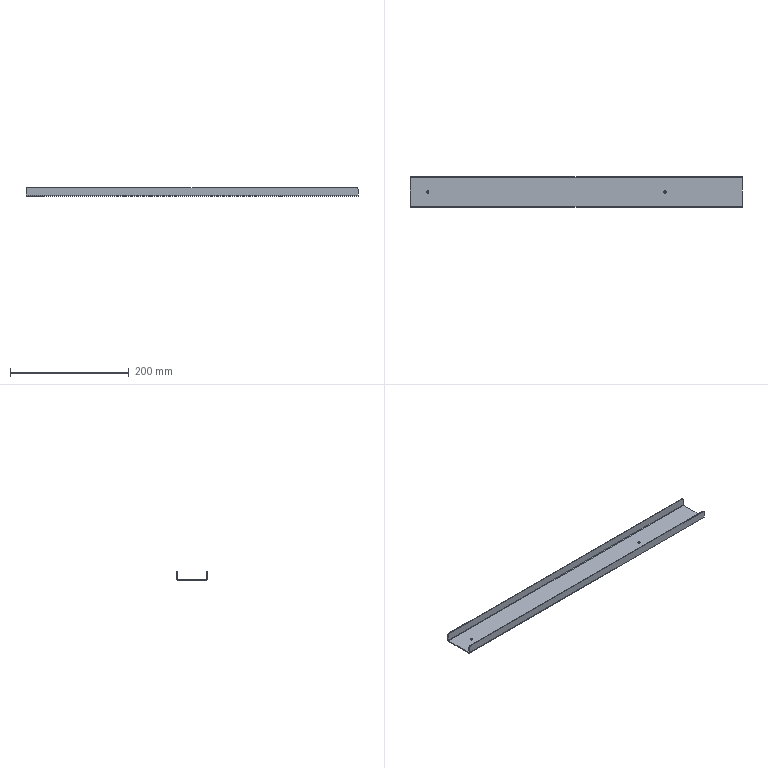Part | SolidWorks | features ICE 2, EdgeFlange 1, Fillet 1, FlatPattern 1, HoleWzd 1, LPattern 1, SMBaseFlange 1, SheetMetal 1 | 1 solid | 30 faces | box 560 x 52 x 15 mm | volume 65239 mm3 | plane 18 | cylinder 12 | commonest cylinder face diameters 4 x4 6 x4 1.473 x2 4.473 x2
STEP:
#1=CARTESIAN_POINT('',(148.,0.,-1.5));
#2=VERTEX_POINT('',#1);
#3=CARTESIAN_POINT('',(152.,0.,-1.5));
#4=VERTEX_POINT('',#3);
#5=CARTESIAN_POINT('',(150.,0.,-1.5));
#6=DIRECTION('',(0.,0.,1.));
#7=DIRECTION('',(1.,0.,0.));
#8=AXIS2_PLACEMENT_3D('',#5,#6,#7);
#9=CIRCLE('',#8,2.);
#10=EDGE_CURVE('',#2,#4,#9,.T.);
#11=ORIENTED_EDGE('',*,*,#10,.F.);
#12=CARTESIAN_POINT('',(148.,0.,0.));
#13=VERTEX_POINT('',#12);
#14=CARTESIAN_POINT('',(148.,0.,-1.5));
#15=DIRECTION('',(0.,0.,1.));
#16=VECTOR('',#15,1000.);
#17=LINE('',#14,#16);
#18=EDGE_CURVE('',#2,#13,#17,.T.);
#19=ORIENTED_EDGE('',*,*,#18,.T.);
#20=CARTESIAN_POINT('',(152.,0.,0.));
#21=VERTEX_POINT('',#20);
#22=CARTESIAN_POINT('',(150.,0.,0.));
#23=DIRECTION('',(0.,0.,1.));
#24=DIRECTION('',(1.,0.,0.));
#25=AXIS2_PLACEMENT_3D('',#22,#23,#24);
#26=CIRCLE('',#25,2.);
#27=EDGE_CURVE('',#13,#21,#26,.T.);
#28=ORIENTED_EDGE('',*,*,#27,.T.);
#29=CARTESIAN_POINT('',(152.,0.,-1.5));
#30=DIRECTION('',(0.,0.,1.));
#31=VECTOR('',#30,1000.);
#32=LINE('',#29,#31);
#33=EDGE_CURVE('',#4,#21,#32,.T.);
#34=ORIENTED_EDGE('',*,*,#33,.F.);
#35=EDGE_LOOP('',(#11,#19,#28,#34));
#36=FACE_OUTER_BOUND('',#35,.T.);
#37=CARTESIAN_POINT('',(150.,0.,-1.5));
#38=DIRECTION('',(0.,0.,1.));
#39=DIRECTION('',(1.,0.,0.));
#40=AXIS2_PLACEMENT_3D('',#37,#38,#39);
#41=CYLINDRICAL_SURFACE('',#40,2.);
#42=ADVANCED_FACE('',(#36),#41,.F.);
#43=CARTESIAN_POINT('',(-252.,0.,-1.5));
#44=VERTEX_POINT('',#43);
#45=CARTESIAN_POINT('',(-248.,0.,-1.5));
#46=VERTEX_POINT('',#45);
#47=CARTESIAN_POINT('',(-250.,0.,-1.5));
#48=DIRECTION('',(0.,0.,1.));
#49=DIRECTION('',(1.,0.,0.));
#50=AXIS2_PLACEMENT_3D('',#47,#48,#49);
#51=CIRCLE('',#50,2.);
#52=EDGE_CURVE('',#44,#46,#51,.T.);
#53=ORIENTED_EDGE('',*,*,#52,.F.);
#54=CARTESIAN_POINT('',(-252.,0.,0.));
#55=VERTEX_POINT('',#54);
#56=CARTESIAN_POINT('',(-252.,0.,-1.5));
#57=DIRECTION('',(0.,0.,1.));
#58=VECTOR('',#57,1000.);
#59=LINE('',#56,#58);
#60=EDGE_CURVE('',#44,#55,#59,.T.);
#61=ORIENTED_EDGE('',*,*,#60,.T.);
#62=CARTESIAN_POINT('',(-248.,0.,0.));
#63=VERTEX_POINT('',#62);
#64=CARTESIAN_POINT('',(-250.,0.,0.));
#65=DIRECTION('',(0.,0.,1.));
#66=DIRECTION('',(1.,0.,0.));
#67=AXIS2_PLACEMENT_3D('',#64,#65,#66);
#68=CIRCLE('',#67,2.);
#69=EDGE_CURVE('',#55,#63,#68,.T.);
#70=ORIENTED_EDGE('',*,*,#69,.T.);
#71=CARTESIAN_POINT('',(-248.,0.,-1.5));
#72=DIRECTION('',(0.,0.,1.));
#73=VECTOR('',#72,1000.);
#74=LINE('',#71,#73);
#75=EDGE_CURVE('',#46,#63,#74,.T.);
#76=ORIENTED_EDGE('',*,*,#75,.F.);
#77=EDGE_LOOP('',(#53,#61,#70,#76));
#78=FACE_OUTER_BOUND('',#77,.T.);
#79=CARTESIAN_POINT('',(-250.,0.,-1.5));
#80=DIRECTION('',(0.,0.,1.));
#81=DIRECTION('',(1.,0.,0.));
#82=AXIS2_PLACEMENT_3D('',#79,#80,#81);
#83=CYLINDRICAL_SURFACE('',#82,2.);
#84=ADVANCED_FACE('',(#78),#83,.F.);
#85=CARTESIAN_POINT('',(150.,0.,-1.5));
#86=DIRECTION('',(0.,0.,1.));
#87=DIRECTION('',(1.,0.,0.));
#88=AXIS2_PLACEMENT_3D('',#85,#86,#87);
#89=CIRCLE('',#88,2.);
#90=EDGE_CURVE('',#4,#2,#89,.T.);
#91=ORIENTED_EDGE('',*,*,#90,.T.);
#92=ORIENTED_EDGE('',*,*,#10,.T.);
#93=EDGE_LOOP('',(#91,#92));
#94=FACE_BOUND('',#93,.T.);
#95=CARTESIAN_POINT('',(-250.,0.,-1.5));
#96=DIRECTION('',(0.,0.,1.));
#97=DIRECTION('',(1.,0.,0.));
#98=AXIS2_PLACEMENT_3D('',#95,#96,#97);
#99=CIRCLE('',#98,2.);
#100=EDGE_CURVE('',#46,#44,#99,.T.);
#101=ORIENTED_EDGE('',*,*,#100,.T.);
#102=ORIENTED_EDGE('',*,*,#52,.T.);
#103=EDGE_LOOP('',(#101,#102));
#104=FACE_BOUND('',#103,.T.);
#105=CARTESIAN_POINT('',(280.,-23.763,-1.5));
#106=VERTEX_POINT('',#105);
#107=CARTESIAN_POINT('',(280.,23.763,-1.5));
#108=VERTEX_POINT('',#107);
#109=CARTESIAN_POINT('',(280.,-26.,-1.5));
#110=DIRECTION('',(0.,1.,0.));
#111=VECTOR('',#110,1000.);
#112=LINE('',#109,#111);
#113=EDGE_CURVE('',#106,#108,#112,.T.);
#114=ORIENTED_EDGE('',*,*,#113,.F.);
#115=CARTESIAN_POINT('',(-280.,-23.763,-1.5));
#116=VERTEX_POINT('',#115);
#117=CARTESIAN_POINT('',(280.,-23.763,-1.5));
#118=DIRECTION('',(-1.,0.,0.));
#119=VECTOR('',#118,1000.);
#120=LINE('',#117,#119);
#121=EDGE_CURVE('',#106,#116,#120,.T.);
#122=ORIENTED_EDGE('',*,*,#121,.T.);
#123=CARTESIAN_POINT('',(-280.,23.763,-1.5));
#124=VERTEX_POINT('',#123);
#125=CARTESIAN_POINT('',(-280.,-26.,-1.5));
#126=DIRECTION('',(0.,-1.,0.));
#127=VECTOR('',#126,1000.);
#128=LINE('',#125,#127);
#129=EDGE_CURVE('',#124,#116,#128,.T.);
#130=ORIENTED_EDGE('',*,*,#129,.F.);
#131=CARTESIAN_POINT('',(-280.,23.763,-1.5));
#132=DIRECTION('',(1.,0.,0.));
#133=VECTOR('',#132,1000.);
#134=LINE('',#131,#133);
#135=EDGE_CURVE('',#124,#108,#134,.T.);
#136=ORIENTED_EDGE('',*,*,#135,.T.);
#137=EDGE_LOOP('',(#114,#122,#130,#136));
#138=FACE_OUTER_BOUND('',#137,.T.);
#139=CARTESIAN_POINT('',(0.,0.,-1.5));
#140=DIRECTION('',(0.,0.,-1.));
#141=DIRECTION('',(-1.,0.,0.));
#142=AXIS2_PLACEMENT_3D('',#139,#140,#141);
#143=PLANE('',#142);
#144=ADVANCED_FACE('',(#94,#104,#138),#143,.T.);
#145=CARTESIAN_POINT('',(150.,0.,0.));
#146=DIRECTION('',(0.,0.,1.));
#147=DIRECTION('',(1.,0.,0.));
#148=AXIS2_PLACEMENT_3D('',#145,#146,#147);
#149=CIRCLE('',#148,2.);
#150=EDGE_CURVE('',#21,#13,#149,.T.);
#151=ORIENTED_EDGE('',*,*,#150,.F.);
#152=ORIENTED_EDGE('',*,*,#27,.F.);
#153=EDGE_LOOP('',(#151,#152));
#154=FACE_BOUND('',#153,.T.);
#155=CARTESIAN_POINT('',(-250.,0.,0.));
#156=DIRECTION('',(0.,0.,1.));
#157=DIRECTION('',(1.,0.,0.));
#158=AXIS2_PLACEMENT_3D('',#155,#156,#157);
#159=CIRCLE('',#158,2.);
#160=EDGE_CURVE('',#63,#55,#159,.T.);
#161=ORIENTED_EDGE('',*,*,#160,.F.);
#162=ORIENTED_EDGE('',*,*,#69,.F.);
#163=EDGE_LOOP('',(#161,#162));
#164=FACE_BOUND('',#163,.T.);
#165=CARTESIAN_POINT('',(280.,-23.763,0.));
#166=VERTEX_POINT('',#165);
#167=CARTESIAN_POINT('',(-280.,-23.763,0.));
#168=VERTEX_POINT('',#167);
#169=CARTESIAN_POINT('',(280.,-23.763,0.));
#170=DIRECTION('',(-1.,0.,0.));
#171=VECTOR('',#170,1000.);
#172=LINE('',#169,#171);
#173=EDGE_CURVE('',#166,#168,#172,.T.);
#174=ORIENTED_EDGE('',*,*,#173,.F.);
#175=CARTESIAN_POINT('',(280.,23.763,0.));
#176=VERTEX_POINT('',#175);
#177=CARTESIAN_POINT('',(280.,-26.,0.));
#178=DIRECTION('',(0.,1.,0.));
#179=VECTOR('',#178,1000.);
#180=LINE('',#177,#179);
#181=EDGE_CURVE('',#166,#176,#180,.T.);
#182=ORIENTED_EDGE('',*,*,#181,.T.);
#183=CARTESIAN_POINT('',(-280.,23.763,0.));
#184=VERTEX_POINT('',#183);
#185=CARTESIAN_POINT('',(-280.,23.763,0.));
#186=DIRECTION('',(1.,0.,0.));
#187=VECTOR('',#186,1000.);
#188=LINE('',#185,#187);
#189=EDGE_CURVE('',#184,#176,#188,.T.);
#190=ORIENTED_EDGE('',*,*,#189,.F.);
#191=CARTESIAN_POINT('',(-280.,-26.,0.));
#192=DIRECTION('',(0.,-1.,0.));
#193=VECTOR('',#192,1000.);
#194=LINE('',#191,#193);
#195=EDGE_CURVE('',#184,#168,#194,.T.);
#196=ORIENTED_EDGE('',*,*,#195,.T.);
#197=EDGE_LOOP('',(#174,#182,#190,#196));
#198=FACE_OUTER_BOUND('',#197,.T.);
#199=CARTESIAN_POINT('',(0.,0.,0.));
#200=DIRECTION('',(0.,0.,-1.));
#201=DIRECTION('',(-1.,0.,0.));
#202=AXIS2_PLACEMENT_3D('',#199,#200,#201);
#203=PLANE('',#202);
#204=ADVANCED_FACE('',(#154,#164,#198),#203,.F.);
#205=ORIENTED_EDGE('',*,*,#181,.F.);
#206=CARTESIAN_POINT('',(280.,-23.763,0.));
#207=DIRECTION('',(0.,0.,-1.));
#208=VECTOR('',#207,1000.);
#209=LINE('',#206,#208);
#210=EDGE_CURVE('',#166,#106,#209,.T.);
#211=ORIENTED_EDGE('',*,*,#210,.T.);
#212=ORIENTED_EDGE('',*,*,#113,.T.);
#213=CARTESIAN_POINT('',(280.,23.763,0.));
#214=DIRECTION('',(0.,0.,-1.));
#215=VECTOR('',#214,1000.);
#216=LINE('',#213,#215);
#217=EDGE_CURVE('',#176,#108,#216,.T.);
#218=ORIENTED_EDGE('',*,*,#217,.F.);
#219=EDGE_LOOP('',(#205,#211,#212,#218));
#220=FACE_OUTER_BOUND('',#219,.T.);
#221=CARTESIAN_POINT('',(280.,-26.,-1.5));
#222=DIRECTION('',(1.,0.,0.));
#223=DIRECTION('',(0.,0.,-1.));
#224=AXIS2_PLACEMENT_3D('',#221,#222,#223);
#225=PLANE('',#224);
#226=ADVANCED_FACE('',(#220),#225,.T.);
#227=CARTESIAN_POINT('',(-280.,-23.763,0.));
#228=DIRECTION('',(0.,0.,-1.));
#229=VECTOR('',#228,1000.);
#230=LINE('',#227,#229);
#231=EDGE_CURVE('',#168,#116,#230,.T.);
#232=ORIENTED_EDGE('',*,*,#231,.F.);
#233=ORIENTED_EDGE('',*,*,#195,.F.);
#234=CARTESIAN_POINT('',(-280.,23.763,0.));
#235=DIRECTION('',(0.,0.,-1.));
#236=VECTOR('',#235,1000.);
#237=LINE('',#234,#236);
#238=EDGE_CURVE('',#184,#124,#237,.T.);
#239=ORIENTED_EDGE('',*,*,#238,.T.);
#240=ORIENTED_EDGE('',*,*,#129,.T.);
#241=EDGE_LOOP('',(#232,#233,#239,#240));
#242=FACE_OUTER_BOUND('',#241,.T.);
#243=CARTESIAN_POINT('',(-280.,-26.,-1.5));
#244=DIRECTION('',(-1.,0.,0.));
#245=DIRECTION('',(0.,0.,1.));
#246=AXIS2_PLACEMENT_3D('',#243,#244,#245);
#247=PLANE('',#246);
#248=ADVANCED_FACE('',(#242),#247,.T.);
#249=CARTESIAN_POINT('',(280.,24.5,0.7366));
#250=VERTEX_POINT('',#249);
#251=CARTESIAN_POINT('',(280.,26.,0.7366));
#252=VERTEX_POINT('',#251);
#253=CARTESIAN_POINT('',(280.,26.,0.7366));
#254=DIRECTION('',(0.,1.,0.));
#255=VECTOR('',#254,1000.);
#256=LINE('',#253,#255);
#257=EDGE_CURVE('',#250,#252,#256,.T.);
#258=ORIENTED_EDGE('',*,*,#257,.F.);
#259=CARTESIAN_POINT('',(280.,23.763,0.7366));
#260=DIRECTION('',(1.,0.,0.));
#261=DIRECTION('',(0.,0.,1.));
#262=AXIS2_PLACEMENT_3D('',#259,#260,#261);
#263=CIRCLE('',#262,0.7366);
#264=EDGE_CURVE('',#176,#250,#263,.T.);
#265=ORIENTED_EDGE('',*,*,#264,.F.);
#266=ORIENTED_EDGE('',*,*,#217,.T.);
#267=CARTESIAN_POINT('',(280.,23.763,0.7366));
#268=DIRECTION('',(1.,0.,0.));
#269=DIRECTION('',(0.,0.,1.));
#270=AXIS2_PLACEMENT_3D('',#267,#268,#269);
#271=CIRCLE('',#270,2.237);
#272=EDGE_CURVE('',#108,#252,#271,.T.);
#273=ORIENTED_EDGE('',*,*,#272,.T.);
#274=EDGE_LOOP('',(#258,#265,#266,#273));
#275=FACE_OUTER_BOUND('',#274,.T.);
#276=CARTESIAN_POINT('',(280.,23.763,0.7366));
#277=DIRECTION('',(1.,0.,0.));
#278=DIRECTION('',(0.,0.,-1.));
#279=AXIS2_PLACEMENT_3D('',#276,#277,#278);
#280=PLANE('',#279);
#281=ADVANCED_FACE('',(#275),#280,.T.);
#282=CARTESIAN_POINT('',(-280.,24.5,0.7366));
#283=VERTEX_POINT('',#282);
#284=CARTESIAN_POINT('',(-280.,23.763,0.7366));
#285=DIRECTION('',(-1.,0.,0.));
#286=DIRECTION('',(0.,0.,1.));
#287=AXIS2_PLACEMENT_3D('',#284,#285,#286);
#288=CIRCLE('',#287,0.7366);
#289=EDGE_CURVE('',#283,#184,#288,.T.);
#290=ORIENTED_EDGE('',*,*,#289,.F.);
#291=CARTESIAN_POINT('',(-280.,26.,0.7366));
#292=VERTEX_POINT('',#291);
#293=CARTESIAN_POINT('',(-280.,24.5,0.7366));
#294=DIRECTION('',(0.,1.,0.));
#295=VECTOR('',#294,1000.);
#296=LINE('',#293,#295);
#297=EDGE_CURVE('',#283,#292,#296,.T.);
#298=ORIENTED_EDGE('',*,*,#297,.T.);
#299=CARTESIAN_POINT('',(-280.,23.763,0.7366));
#300=DIRECTION('',(-1.,0.,0.));
#301=DIRECTION('',(0.,0.,1.));
#302=AXIS2_PLACEMENT_3D('',#299,#300,#301);
#303=CIRCLE('',#302,2.237);
#304=EDGE_CURVE('',#292,#124,#303,.T.);
#305=ORIENTED_EDGE('',*,*,#304,.T.);
#306=ORIENTED_EDGE('',*,*,#238,.F.);
#307=EDGE_LOOP('',(#290,#298,#305,#306));
#308=FACE_OUTER_BOUND('',#307,.T.);
#309=CARTESIAN_POINT('',(-280.,23.763,0.7366));
#310=DIRECTION('',(1.,0.,0.));
#311=DIRECTION('',(0.,0.,-1.));
#312=AXIS2_PLACEMENT_3D('',#309,#310,#311);
#313=PLANE('',#312);
#314=ADVANCED_FACE('',(#308),#313,.F.);
#315=ORIENTED_EDGE('',*,*,#135,.F.);
#316=ORIENTED_EDGE('',*,*,#304,.F.);
#317=CARTESIAN_POINT('',(280.,26.,0.7366));
#318=DIRECTION('',(1.,0.,0.));
#319=VECTOR('',#318,1000.);
#320=LINE('',#317,#319);
#321=EDGE_CURVE('',#292,#252,#320,.T.);
#322=ORIENTED_EDGE('',*,*,#321,.T.);
#323=ORIENTED_EDGE('',*,*,#272,.F.);
#324=EDGE_LOOP('',(#315,#316,#322,#323));
#325=FACE_OUTER_BOUND('',#324,.T.);
#326=CARTESIAN_POINT('',(-280.,23.763,0.7366));
#327=DIRECTION('',(-1.,0.,0.));
#328=DIRECTION('',(0.,1.,0.));
#329=AXIS2_PLACEMENT_3D('',#326,#327,#328);
#330=CYLINDRICAL_SURFACE('',#329,2.237);
#331=ADVANCED_FACE('',(#325),#330,.T.);
#332=ORIENTED_EDGE('',*,*,#189,.T.);
#333=ORIENTED_EDGE('',*,*,#264,.T.);
#334=CARTESIAN_POINT('',(280.,24.5,0.7366));
#335=DIRECTION('',(-1.,0.,0.));
#336=VECTOR('',#335,1000.);
#337=LINE('',#334,#336);
#338=EDGE_CURVE('',#250,#283,#337,.T.);
#339=ORIENTED_EDGE('',*,*,#338,.T.);
#340=ORIENTED_EDGE('',*,*,#289,.T.);
#341=EDGE_LOOP('',(#332,#333,#339,#340));
#342=FACE_OUTER_BOUND('',#341,.T.);
#343=CARTESIAN_POINT('',(-280.,23.763,0.7366));
#344=DIRECTION('',(-1.,0.,0.));
#345=DIRECTION('',(0.,1.,0.));
#346=AXIS2_PLACEMENT_3D('',#343,#344,#345);
#347=CYLINDRICAL_SURFACE('',#346,0.7366);
#348=ADVANCED_FACE('',(#342),#347,.F.);
#349=CARTESIAN_POINT('',(280.,26.,10.5));
#350=VERTEX_POINT('',#349);
#351=CARTESIAN_POINT('',(280.,26.,0.));
#352=DIRECTION('',(0.,0.,-1.));
#353=VECTOR('',#352,1000.);
#354=LINE('',#351,#353);
#355=EDGE_CURVE('',#350,#252,#354,.T.);
#356=ORIENTED_EDGE('',*,*,#355,.F.);
#357=CARTESIAN_POINT('',(280.,24.5,10.5));
#358=VERTEX_POINT('',#357);
#359=CARTESIAN_POINT('',(280.,26.,10.5));
#360=DIRECTION('',(0.,-1.,0.));
#361=VECTOR('',#360,1000.);
#362=LINE('',#359,#361);
#363=EDGE_CURVE('',#350,#358,#362,.T.);
#364=ORIENTED_EDGE('',*,*,#363,.T.);
#365=CARTESIAN_POINT('',(280.,24.5,0.));
#366=DIRECTION('',(0.,0.,-1.));
#367=VECTOR('',#366,1000.);
#368=LINE('',#365,#367);
#369=EDGE_CURVE('',#358,#250,#368,.T.);
#370=ORIENTED_EDGE('',*,*,#369,.T.);
#371=ORIENTED_EDGE('',*,*,#257,.T.);
#372=EDGE_LOOP('',(#356,#364,#370,#371));
#373=FACE_OUTER_BOUND('',#372,.T.);
#374=CARTESIAN_POINT('',(280.,26.,0.));
#375=DIRECTION('',(-1.,0.,0.));
#376=DIRECTION('',(0.,0.,1.));
#377=AXIS2_PLACEMENT_3D('',#374,#375,#376);
#378=PLANE('',#377);
#379=ADVANCED_FACE('',(#373),#378,.F.);
#380=CARTESIAN_POINT('',(-280.,24.5,10.5));
#381=VERTEX_POINT('',#380);
#382=CARTESIAN_POINT('',(-280.,24.5,13.5));
#383=DIRECTION('',(0.,0.,1.));
#384=VECTOR('',#383,1000.);
#385=LINE('',#382,#384);
#386=EDGE_CURVE('',#283,#381,#385,.T.);
#387=ORIENTED_EDGE('',*,*,#386,.T.);
#388=CARTESIAN_POINT('',(-280.,26.,10.5));
#389=VERTEX_POINT('',#388);
#390=CARTESIAN_POINT('',(-280.,26.,10.5));
#391=DIRECTION('',(0.,1.,0.));
#392=VECTOR('',#391,1000.);
#393=LINE('',#390,#392);
#394=EDGE_CURVE('',#381,#389,#393,.T.);
#395=ORIENTED_EDGE('',*,*,#394,.T.);
#396=CARTESIAN_POINT('',(-280.,26.,0.));
#397=DIRECTION('',(0.,0.,1.));
#398=VECTOR('',#397,1000.);
#399=LINE('',#396,#398);
#400=EDGE_CURVE('',#292,#389,#399,.T.);
#401=ORIENTED_EDGE('',*,*,#400,.F.);
#402=ORIENTED_EDGE('',*,*,#297,.F.);
#403=EDGE_LOOP('',(#387,#395,#401,#402));
#404=FACE_OUTER_BOUND('',#403,.T.);
#405=CARTESIAN_POINT('',(-280.,26.,13.5));
#406=DIRECTION('',(1.,0.,0.));
#407=DIRECTION('',(0.,0.,-1.));
#408=AXIS2_PLACEMENT_3D('',#405,#406,#407);
#409=PLANE('',#408);
#410=ADVANCED_FACE('',(#404),#409,.F.);
#411=CARTESIAN_POINT('',(-277.,26.,13.5));
#412=VERTEX_POINT('',#411);
#413=CARTESIAN_POINT('',(277.,26.,13.5));
#414=VERTEX_POINT('',#413);
#415=CARTESIAN_POINT('',(0.,26.,13.5));
#416=DIRECTION('',(1.,0.,0.));
#417=VECTOR('',#416,1000.);
#418=LINE('',#415,#417);
#419=EDGE_CURVE('',#412,#414,#418,.T.);
#420=ORIENTED_EDGE('',*,*,#419,.T.);
#421=CARTESIAN_POINT('',(277.,26.,10.5));
#422=DIRECTION('',(0.,1.,0.));
#423=DIRECTION('',(0.,0.,-1.));
#424=AXIS2_PLACEMENT_3D('',#421,#422,#423);
#425=CIRCLE('',#424,3.);
#426=EDGE_CURVE('',#414,#350,#425,.T.);
#427=ORIENTED_EDGE('',*,*,#426,.T.);
#428=ORIENTED_EDGE('',*,*,#355,.T.);
#429=ORIENTED_EDGE('',*,*,#321,.F.);
#430=ORIENTED_EDGE('',*,*,#400,.T.);
#431=CARTESIAN_POINT('',(-277.,26.,10.5));
#432=DIRECTION('',(0.,1.,0.));
#433=DIRECTION('',(0.,0.,-1.));
#434=AXIS2_PLACEMENT_3D('',#431,#432,#433);
#435=CIRCLE('',#434,3.);
#436=EDGE_CURVE('',#389,#412,#435,.T.);
#437=ORIENTED_EDGE('',*,*,#436,.T.);
#438=EDGE_LOOP('',(#420,#427,#428,#429,#430,#437));
#439=FACE_OUTER_BOUND('',#438,.T.);
#440=CARTESIAN_POINT('',(0.,26.,0.));
#441=DIRECTION('',(0.,-1.,0.));
#442=DIRECTION('',(0.,0.,-1.));
#443=AXIS2_PLACEMENT_3D('',#440,#441,#442);
#444=PLANE('',#443);
#445=ADVANCED_FACE('',(#439),#444,.F.);
#446=ORIENTED_EDGE('',*,*,#369,.F.);
#447=CARTESIAN_POINT('',(277.,24.5,13.5));
#448=VERTEX_POINT('',#447);
#449=CARTESIAN_POINT('',(277.,24.5,10.5));
#450=DIRECTION('',(0.,-1.,0.));
#451=DIRECTION('',(0.,0.,-1.));
#452=AXIS2_PLACEMENT_3D('',#449,#450,#451);
#453=CIRCLE('',#452,3.);
#454=EDGE_CURVE('',#358,#448,#453,.T.);
#455=ORIENTED_EDGE('',*,*,#454,.T.);
#456=CARTESIAN_POINT('',(-277.,24.5,13.5));
#457=VERTEX_POINT('',#456);
#458=CARTESIAN_POINT('',(280.,24.5,13.5));
#459=DIRECTION('',(1.,0.,0.));
#460=VECTOR('',#459,1000.);
#461=LINE('',#458,#460);
#462=EDGE_CURVE('',#457,#448,#461,.T.);
#463=ORIENTED_EDGE('',*,*,#462,.F.);
#464=CARTESIAN_POINT('',(-277.,24.5,10.5));
#465=DIRECTION('',(0.,-1.,0.));
#466=DIRECTION('',(0.,0.,-1.));
#467=AXIS2_PLACEMENT_3D('',#464,#465,#466);
#468=CIRCLE('',#467,3.);
#469=EDGE_CURVE('',#457,#381,#468,.T.);
#470=ORIENTED_EDGE('',*,*,#469,.T.);
#471=ORIENTED_EDGE('',*,*,#386,.F.);
#472=ORIENTED_EDGE('',*,*,#338,.F.);
#473=EDGE_LOOP('',(#446,#455,#463,#470,#471,#472));
#474=FACE_OUTER_BOUND('',#473,.T.);
#475=CARTESIAN_POINT('',(0.,24.5,0.));
#476=DIRECTION('',(0.,-1.,0.));
#477=DIRECTION('',(0.,0.,-1.));
#478=AXIS2_PLACEMENT_3D('',#475,#476,#477);
#479=PLANE('',#478);
#480=ADVANCED_FACE('',(#474),#479,.T.);
#481=ORIENTED_EDGE('',*,*,#462,.T.);
#482=CARTESIAN_POINT('',(277.,26.,13.5));
#483=DIRECTION('',(0.,1.,0.));
#484=VECTOR('',#483,1000.);
#485=LINE('',#482,#484);
#486=EDGE_CURVE('',#448,#414,#485,.T.);
#487=ORIENTED_EDGE('',*,*,#486,.T.);
#488=ORIENTED_EDGE('',*,*,#419,.F.);
#489=CARTESIAN_POINT('',(-277.,26.,13.5));
#490=DIRECTION('',(0.,-1.,0.));
#491=VECTOR('',#490,1000.);
#492=LINE('',#489,#491);
#493=EDGE_CURVE('',#412,#457,#492,.T.);
#494=ORIENTED_EDGE('',*,*,#493,.T.);
#495=EDGE_LOOP('',(#481,#487,#488,#494));
#496=FACE_OUTER_BOUND('',#495,.T.);
#497=CARTESIAN_POINT('',(280.,26.,13.5));
#498=DIRECTION('',(0.,0.,-1.));
#499=DIRECTION('',(0.,1.,0.));
#500=AXIS2_PLACEMENT_3D('',#497,#498,#499);
#501=PLANE('',#500);
#502=ADVANCED_FACE('',(#496),#501,.F.);
#503=CARTESIAN_POINT('',(-280.,-24.5,0.7366));
#504=VERTEX_POINT('',#503);
#505=CARTESIAN_POINT('',(-280.,-26.,0.7366));
#506=VERTEX_POINT('',#505);
#507=CARTESIAN_POINT('',(-280.,-26.,0.7366));
#508=DIRECTION('',(0.,-1.,0.));
#509=VECTOR('',#508,1000.);
#510=LINE('',#507,#509);
#511=EDGE_CURVE('',#504,#506,#510,.T.);
#512=ORIENTED_EDGE('',*,*,#511,.F.);
#513=CARTESIAN_POINT('',(-280.,-23.763,0.7366));
#514=DIRECTION('',(-1.,0.,0.));
#515=DIRECTION('',(0.,0.,-1.));
#516=AXIS2_PLACEMENT_3D('',#513,#514,#515);
#517=CIRCLE('',#516,0.7366);
#518=EDGE_CURVE('',#168,#504,#517,.T.);
#519=ORIENTED_EDGE('',*,*,#518,.F.);
#520=ORIENTED_EDGE('',*,*,#231,.T.);
#521=CARTESIAN_POINT('',(-280.,-23.763,0.7366));
#522=DIRECTION('',(-1.,0.,0.));
#523=DIRECTION('',(0.,0.,-1.));
#524=AXIS2_PLACEMENT_3D('',#521,#522,#523);
#525=CIRCLE('',#524,2.237);
#526=EDGE_CURVE('',#116,#506,#525,.T.);
#527=ORIENTED_EDGE('',*,*,#526,.T.);
#528=EDGE_LOOP('',(#512,#519,#520,#527));
#529=FACE_OUTER_BOUND('',#528,.T.);
#530=CARTESIAN_POINT('',(-280.,-23.763,0.7366));
#531=DIRECTION('',(-1.,0.,0.));
#532=DIRECTION('',(0.,0.,1.));
#533=AXIS2_PLACEMENT_3D('',#530,#531,#532);
#534=PLANE('',#533);
#535=ADVANCED_FACE('',(#529),#534,.T.);
#536=CARTESIAN_POINT('',(280.,-24.5,0.7366));
#537=VERTEX_POINT('',#536);
#538=CARTESIAN_POINT('',(280.,-23.763,0.7366));
#539=DIRECTION('',(1.,0.,0.));
#540=DIRECTION('',(0.,0.,-1.));
#541=AXIS2_PLACEMENT_3D('',#538,#539,#540);
#542=CIRCLE('',#541,0.7366);
#543=EDGE_CURVE('',#537,#166,#542,.T.);
#544=ORIENTED_EDGE('',*,*,#543,.F.);
#545=CARTESIAN_POINT('',(280.,-26.,0.7366));
#546=VERTEX_POINT('',#545);
#547=CARTESIAN_POINT('',(280.,-24.5,0.7366));
#548=DIRECTION('',(0.,-1.,0.));
#549=VECTOR('',#548,1000.);
#550=LINE('',#547,#549);
#551=EDGE_CURVE('',#537,#546,#550,.T.);
#552=ORIENTED_EDGE('',*,*,#551,.T.);
#553=CARTESIAN_POINT('',(280.,-23.763,0.7366));
#554=DIRECTION('',(1.,0.,0.));
#555=DIRECTION('',(0.,0.,-1.));
#556=AXIS2_PLACEMENT_3D('',#553,#554,#555);
#557=CIRCLE('',#556,2.237);
#558=EDGE_CURVE('',#546,#106,#557,.T.);
#559=ORIENTED_EDGE('',*,*,#558,.T.);
#560=ORIENTED_EDGE('',*,*,#210,.F.);
#561=EDGE_LOOP('',(#544,#552,#559,#560));
#562=FACE_OUTER_BOUND('',#561,.T.);
#563=CARTESIAN_POINT('',(280.,-23.763,0.7366));
#564=DIRECTION('',(-1.,0.,0.));
#565=DIRECTION('',(0.,0.,1.));
#566=AXIS2_PLACEMENT_3D('',#563,#564,#565);
#567=PLANE('',#566);
#568=ADVANCED_FACE('',(#562),#567,.F.);
#569=ORIENTED_EDGE('',*,*,#121,.F.);
#570=ORIENTED_EDGE('',*,*,#558,.F.);
#571=CARTESIAN_POINT('',(-280.,-26.,0.7366));
#572=DIRECTION('',(-1.,0.,0.));
#573=VECTOR('',#572,1000.);
#574=LINE('',#571,#573);
#575=EDGE_CURVE('',#546,#506,#574,.T.);
#576=ORIENTED_EDGE('',*,*,#575,.T.);
#577=ORIENTED_EDGE('',*,*,#526,.F.);
#578=EDGE_LOOP('',(#569,#570,#576,#577));
#579=FACE_OUTER_BOUND('',#578,.T.);
#580=CARTESIAN_POINT('',(280.,-23.763,0.7366));
#581=DIRECTION('',(1.,0.,0.));
#582=DIRECTION('',(0.,-1.,0.));
#583=AXIS2_PLACEMENT_3D('',#580,#581,#582);
#584=CYLINDRICAL_SURFACE('',#583,2.237);
#585=ADVANCED_FACE('',(#579),#584,.T.);
#586=ORIENTED_EDGE('',*,*,#173,.T.);
#587=ORIENTED_EDGE('',*,*,#518,.T.);
#588=CARTESIAN_POINT('',(-280.,-24.5,0.7366));
#589=DIRECTION('',(1.,0.,0.));
#590=VECTOR('',#589,1000.);
#591=LINE('',#588,#590);
#592=EDGE_CURVE('',#504,#537,#591,.T.);
#593=ORIENTED_EDGE('',*,*,#592,.T.);
#594=ORIENTED_EDGE('',*,*,#543,.T.);
#595=EDGE_LOOP('',(#586,#587,#593,#594));
#596=FACE_OUTER_BOUND('',#595,.T.);
#597=CARTESIAN_POINT('',(280.,-23.763,0.7366));
#598=DIRECTION('',(1.,0.,0.));
#599=DIRECTION('',(0.,-1.,0.));
#600=AXIS2_PLACEMENT_3D('',#597,#598,#599);
#601=CYLINDRICAL_SURFACE('',#600,0.7366);
#602=ADVANCED_FACE('',(#596),#601,.F.);
#603=CARTESIAN_POINT('',(-280.,-26.,10.5));
#604=VERTEX_POINT('',#603);
#605=CARTESIAN_POINT('',(-280.,-26.,0.));
#606=DIRECTION('',(0.,0.,-1.));
#607=VECTOR('',#606,1000.);
#608=LINE('',#605,#607);
#609=EDGE_CURVE('',#604,#506,#608,.T.);
#610=ORIENTED_EDGE('',*,*,#609,.F.);
#611=CARTESIAN_POINT('',(-280.,-24.5,10.5));
#612=VERTEX_POINT('',#611);
#613=CARTESIAN_POINT('',(-280.,-26.,10.5));
#614=DIRECTION('',(0.,1.,0.));
#615=VECTOR('',#614,1000.);
#616=LINE('',#613,#615);
#617=EDGE_CURVE('',#604,#612,#616,.T.);
#618=ORIENTED_EDGE('',*,*,#617,.T.);
#619=CARTESIAN_POINT('',(-280.,-24.5,0.));
#620=DIRECTION('',(0.,0.,-1.));
#621=VECTOR('',#620,1000.);
#622=LINE('',#619,#621);
#623=EDGE_CURVE('',#612,#504,#622,.T.);
#624=ORIENTED_EDGE('',*,*,#623,.T.);
#625=ORIENTED_EDGE('',*,*,#511,.T.);
#626=EDGE_LOOP('',(#610,#618,#624,#625));
#627=FACE_OUTER_BOUND('',#626,.T.);
#628=CARTESIAN_POINT('',(-280.,-26.,0.));
#629=DIRECTION('',(1.,0.,0.));
#630=DIRECTION('',(0.,0.,-1.));
#631=AXIS2_PLACEMENT_3D('',#628,#629,#630);
#632=PLANE('',#631);
#633=ADVANCED_FACE('',(#627),#632,.F.);
#634=CARTESIAN_POINT('',(280.,-24.5,10.5));
#635=VERTEX_POINT('',#634);
#636=CARTESIAN_POINT('',(280.,-24.5,13.5));
#637=DIRECTION('',(0.,0.,1.));
#638=VECTOR('',#637,1000.);
#639=LINE('',#636,#638);
#640=EDGE_CURVE('',#537,#635,#639,.T.);
#641=ORIENTED_EDGE('',*,*,#640,.T.);
#642=CARTESIAN_POINT('',(280.,-26.,10.5));
#643=VERTEX_POINT('',#642);
#644=CARTESIAN_POINT('',(280.,-26.,10.5));
#645=DIRECTION('',(0.,-1.,0.));
#646=VECTOR('',#645,1000.);
#647=LINE('',#644,#646);
#648=EDGE_CURVE('',#635,#643,#647,.T.);
#649=ORIENTED_EDGE('',*,*,#648,.T.);
#650=CARTESIAN_POINT('',(280.,-26.,0.));
#651=DIRECTION('',(0.,0.,1.));
#652=VECTOR('',#651,1000.);
#653=LINE('',#650,#652);
#654=EDGE_CURVE('',#546,#643,#653,.T.);
#655=ORIENTED_EDGE('',*,*,#654,.F.);
#656=ORIENTED_EDGE('',*,*,#551,.F.);
#657=EDGE_LOOP('',(#641,#649,#655,#656));
#658=FACE_OUTER_BOUND('',#657,.T.);
#659=CARTESIAN_POINT('',(280.,-26.,13.5));
#660=DIRECTION('',(-1.,0.,0.));
#661=DIRECTION('',(0.,0.,1.));
#662=AXIS2_PLACEMENT_3D('',#659,#660,#661);
#663=PLANE('',#662);
#664=ADVANCED_FACE('',(#658),#663,.F.);
#665=ORIENTED_EDGE('',*,*,#654,.T.);
#666=CARTESIAN_POINT('',(277.,-26.,13.5));
#667=VERTEX_POINT('',#666);
#668=CARTESIAN_POINT('',(277.,-26.,10.5));
#669=DIRECTION('',(0.,-1.,0.));
#670=DIRECTION('',(0.,0.,1.));
#671=AXIS2_PLACEMENT_3D('',#668,#669,#670);
#672=CIRCLE('',#671,3.);
#673=EDGE_CURVE('',#643,#667,#672,.T.);
#674=ORIENTED_EDGE('',*,*,#673,.T.);
#675=CARTESIAN_POINT('',(-277.,-26.,13.5));
#676=VERTEX_POINT('',#675);
#677=CARTESIAN_POINT('',(0.,-26.,13.5));
#678=DIRECTION('',(-1.,0.,0.));
#679=VECTOR('',#678,1000.);
#680=LINE('',#677,#679);
#681=EDGE_CURVE('',#667,#676,#680,.T.);
#682=ORIENTED_EDGE('',*,*,#681,.T.);
#683=CARTESIAN_POINT('',(-277.,-26.,10.5));
#684=DIRECTION('',(0.,-1.,0.));
#685=DIRECTION('',(0.,0.,1.));
#686=AXIS2_PLACEMENT_3D('',#683,#684,#685);
#687=CIRCLE('',#686,3.);
#688=EDGE_CURVE('',#676,#604,#687,.T.);
#689=ORIENTED_EDGE('',*,*,#688,.T.);
#690=ORIENTED_EDGE('',*,*,#609,.T.);
#691=ORIENTED_EDGE('',*,*,#575,.F.);
#692=EDGE_LOOP('',(#665,#674,#682,#689,#690,#691));
#693=FACE_OUTER_BOUND('',#692,.T.);
#694=CARTESIAN_POINT('',(0.,-26.,0.));
#695=DIRECTION('',(0.,1.,0.));
#696=DIRECTION('',(0.,0.,1.));
#697=AXIS2_PLACEMENT_3D('',#694,#695,#696);
#698=PLANE('',#697);
#699=ADVANCED_FACE('',(#693),#698,.F.);
#700=CARTESIAN_POINT('',(277.,-24.5,13.5));
#701=VERTEX_POINT('',#700);
#702=CARTESIAN_POINT('',(-277.,-24.5,13.5));
#703=VERTEX_POINT('',#702);
#704=CARTESIAN_POINT('',(-280.,-24.5,13.5));
#705=DIRECTION('',(-1.,0.,0.));
#706=VECTOR('',#705,1000.);
#707=LINE('',#704,#706);
#708=EDGE_CURVE('',#701,#703,#707,.T.);
#709=ORIENTED_EDGE('',*,*,#708,.F.);
#710=CARTESIAN_POINT('',(277.,-24.5,10.5));
#711=DIRECTION('',(0.,1.,0.));
#712=DIRECTION('',(0.,0.,1.));
#713=AXIS2_PLACEMENT_3D('',#710,#711,#712);
#714=CIRCLE('',#713,3.);
#715=EDGE_CURVE('',#701,#635,#714,.T.);
#716=ORIENTED_EDGE('',*,*,#715,.T.);
#717=ORIENTED_EDGE('',*,*,#640,.F.);
#718=ORIENTED_EDGE('',*,*,#592,.F.);
#719=ORIENTED_EDGE('',*,*,#623,.F.);
#720=CARTESIAN_POINT('',(-277.,-24.5,10.5));
#721=DIRECTION('',(0.,1.,0.));
#722=DIRECTION('',(0.,0.,1.));
#723=AXIS2_PLACEMENT_3D('',#720,#721,#722);
#724=CIRCLE('',#723,3.);
#725=EDGE_CURVE('',#612,#703,#724,.T.);
#726=ORIENTED_EDGE('',*,*,#725,.T.);
#727=EDGE_LOOP('',(#709,#716,#717,#718,#719,#726));
#728=FACE_OUTER_BOUND('',#727,.T.);
#729=CARTESIAN_POINT('',(0.,-24.5,0.));
#730=DIRECTION('',(0.,1.,0.));
#731=DIRECTION('',(0.,0.,1.));
#732=AXIS2_PLACEMENT_3D('',#729,#730,#731);
#733=PLANE('',#732);
#734=ADVANCED_FACE('',(#728),#733,.T.);
#735=ORIENTED_EDGE('',*,*,#681,.F.);
#736=CARTESIAN_POINT('',(277.,-26.,13.5));
#737=DIRECTION('',(0.,1.,0.));
#738=VECTOR('',#737,1000.);
#739=LINE('',#736,#738);
#740=EDGE_CURVE('',#667,#701,#739,.T.);
#741=ORIENTED_EDGE('',*,*,#740,.T.);
#742=ORIENTED_EDGE('',*,*,#708,.T.);
#743=CARTESIAN_POINT('',(-277.,-26.,13.5));
#744=DIRECTION('',(0.,-1.,0.));
#745=VECTOR('',#744,1000.);
#746=LINE('',#743,#745);
#747=EDGE_CURVE('',#703,#676,#746,.T.);
#748=ORIENTED_EDGE('',*,*,#747,.T.);
#749=EDGE_LOOP('',(#735,#741,#742,#748));
#750=FACE_OUTER_BOUND('',#749,.T.);
#751=CARTESIAN_POINT('',(-280.,-26.,13.5));
#752=DIRECTION('',(0.,0.,-1.));
#753=DIRECTION('',(0.,1.,0.));
#754=AXIS2_PLACEMENT_3D('',#751,#752,#753);
#755=PLANE('',#754);
#756=ADVANCED_FACE('',(#750),#755,.F.);
#757=ORIENTED_EDGE('',*,*,#426,.F.);
#758=ORIENTED_EDGE('',*,*,#486,.F.);
#759=ORIENTED_EDGE('',*,*,#454,.F.);
#760=ORIENTED_EDGE('',*,*,#363,.F.);
#761=EDGE_LOOP('',(#757,#758,#759,#760));
#762=FACE_OUTER_BOUND('',#761,.T.);
#763=CARTESIAN_POINT('',(277.,26.,10.5));
#764=DIRECTION('',(0.,-1.,0.));
#765=DIRECTION('',(0.,0.,-1.));
#766=AXIS2_PLACEMENT_3D('',#763,#764,#765);
#767=CYLINDRICAL_SURFACE('',#766,3.);
#768=ADVANCED_FACE('',(#762),#767,.T.);
#769=ORIENTED_EDGE('',*,*,#673,.F.);
#770=ORIENTED_EDGE('',*,*,#648,.F.);
#771=ORIENTED_EDGE('',*,*,#715,.F.);
#772=ORIENTED_EDGE('',*,*,#740,.F.);
#773=EDGE_LOOP('',(#769,#770,#771,#772));
#774=FACE_OUTER_BOUND('',#773,.T.);
#775=CARTESIAN_POINT('',(277.,-26.,10.5));
#776=DIRECTION('',(0.,1.,0.));
#777=DIRECTION('',(0.,0.,1.));
#778=AXIS2_PLACEMENT_3D('',#775,#776,#777);
#779=CYLINDRICAL_SURFACE('',#778,3.);
#780=ADVANCED_FACE('',(#774),#779,.T.);
#781=ORIENTED_EDGE('',*,*,#688,.F.);
#782=ORIENTED_EDGE('',*,*,#747,.F.);
#783=ORIENTED_EDGE('',*,*,#725,.F.);
#784=ORIENTED_EDGE('',*,*,#617,.F.);
#785=EDGE_LOOP('',(#781,#782,#783,#784));
#786=FACE_OUTER_BOUND('',#785,.T.);
#787=CARTESIAN_POINT('',(-277.,-26.,10.5));
#788=DIRECTION('',(0.,1.,0.));
#789=DIRECTION('',(0.,0.,1.));
#790=AXIS2_PLACEMENT_3D('',#787,#788,#789);
#791=CYLINDRICAL_SURFACE('',#790,3.);
#792=ADVANCED_FACE('',(#786),#791,.T.);
#793=ORIENTED_EDGE('',*,*,#436,.F.);
#794=ORIENTED_EDGE('',*,*,#394,.F.);
#795=ORIENTED_EDGE('',*,*,#469,.F.);
#796=ORIENTED_EDGE('',*,*,#493,.F.);
#797=EDGE_LOOP('',(#793,#794,#795,#796));
#798=FACE_OUTER_BOUND('',#797,.T.);
#799=CARTESIAN_POINT('',(-277.,26.,10.5));
#800=DIRECTION('',(0.,-1.,0.));
#801=DIRECTION('',(0.,0.,-1.));
#802=AXIS2_PLACEMENT_3D('',#799,#800,#801);
#803=CYLINDRICAL_SURFACE('',#802,3.);
#804=ADVANCED_FACE('',(#798),#803,.T.);
#805=ORIENTED_EDGE('',*,*,#60,.F.);
#806=ORIENTED_EDGE('',*,*,#100,.F.);
#807=ORIENTED_EDGE('',*,*,#75,.T.);
#808=ORIENTED_EDGE('',*,*,#160,.T.);
#809=EDGE_LOOP('',(#805,#806,#807,#808));
#810=FACE_OUTER_BOUND('',#809,.T.);
#811=CARTESIAN_POINT('',(-250.,0.,-1.5));
#812=DIRECTION('',(0.,0.,1.));
#813=DIRECTION('',(1.,0.,0.));
#814=AXIS2_PLACEMENT_3D('',#811,#812,#813);
#815=CYLINDRICAL_SURFACE('',#814,2.);
#816=ADVANCED_FACE('',(#810),#815,.F.);
#817=ORIENTED_EDGE('',*,*,#18,.F.);
#818=ORIENTED_EDGE('',*,*,#90,.F.);
#819=ORIENTED_EDGE('',*,*,#33,.T.);
#820=ORIENTED_EDGE('',*,*,#150,.T.);
#821=EDGE_LOOP('',(#817,#818,#819,#820));
#822=FACE_OUTER_BOUND('',#821,.T.);
#823=CARTESIAN_POINT('',(150.,0.,-1.5));
#824=DIRECTION('',(0.,0.,1.));
#825=DIRECTION('',(1.,0.,0.));
#826=AXIS2_PLACEMENT_3D('',#823,#824,#825);
#827=CYLINDRICAL_SURFACE('',#826,2.);
#828=ADVANCED_FACE('',(#822),#827,.F.);
#829=CLOSED_SHELL('',(#42,#84,#144,#204,#226,#248,#281,#314,#331,#348,#379,#410,#445,#480,#502,#535,#568,#585,#602,#633,#664,#699,#734,#756,#768,#780,#792,#804,#816,#828));
#830=MANIFOLD_SOLID_BREP('',#829);
#831=CARTESIAN_POINT('',(0.,0.,0.));
#832=DIRECTION('',(0.,0.,1.));
#833=DIRECTION('',(1.,0.,0.));
#834=AXIS2_PLACEMENT_3D('',#831,#832,#833);
#835=(LENGTH_UNIT()NAMED_UNIT(*)SI_UNIT(.MILLI.,.METRE.));
#836=UNCERTAINTY_MEASURE_WITH_UNIT(LENGTH_MEASURE(0.00001),#835,'','');
#837=(NAMED_UNIT(*)PLANE_ANGLE_UNIT()SI_UNIT($,.RADIAN.));
#838=(NAMED_UNIT(*)SI_UNIT($,.STERADIAN.)SOLID_ANGLE_UNIT());
#839=(GEOMETRIC_REPRESENTATION_CONTEXT(3)GLOBAL_UNCERTAINTY_ASSIGNED_CONTEXT((#836))GLOBAL_UNIT_ASSIGNED_CONTEXT((#835,#837,#838))REPRESENTATION_CONTEXT('',''));
#840=ADVANCED_BREP_SHAPE_REPRESENTATION('',(#830,#834),#839);